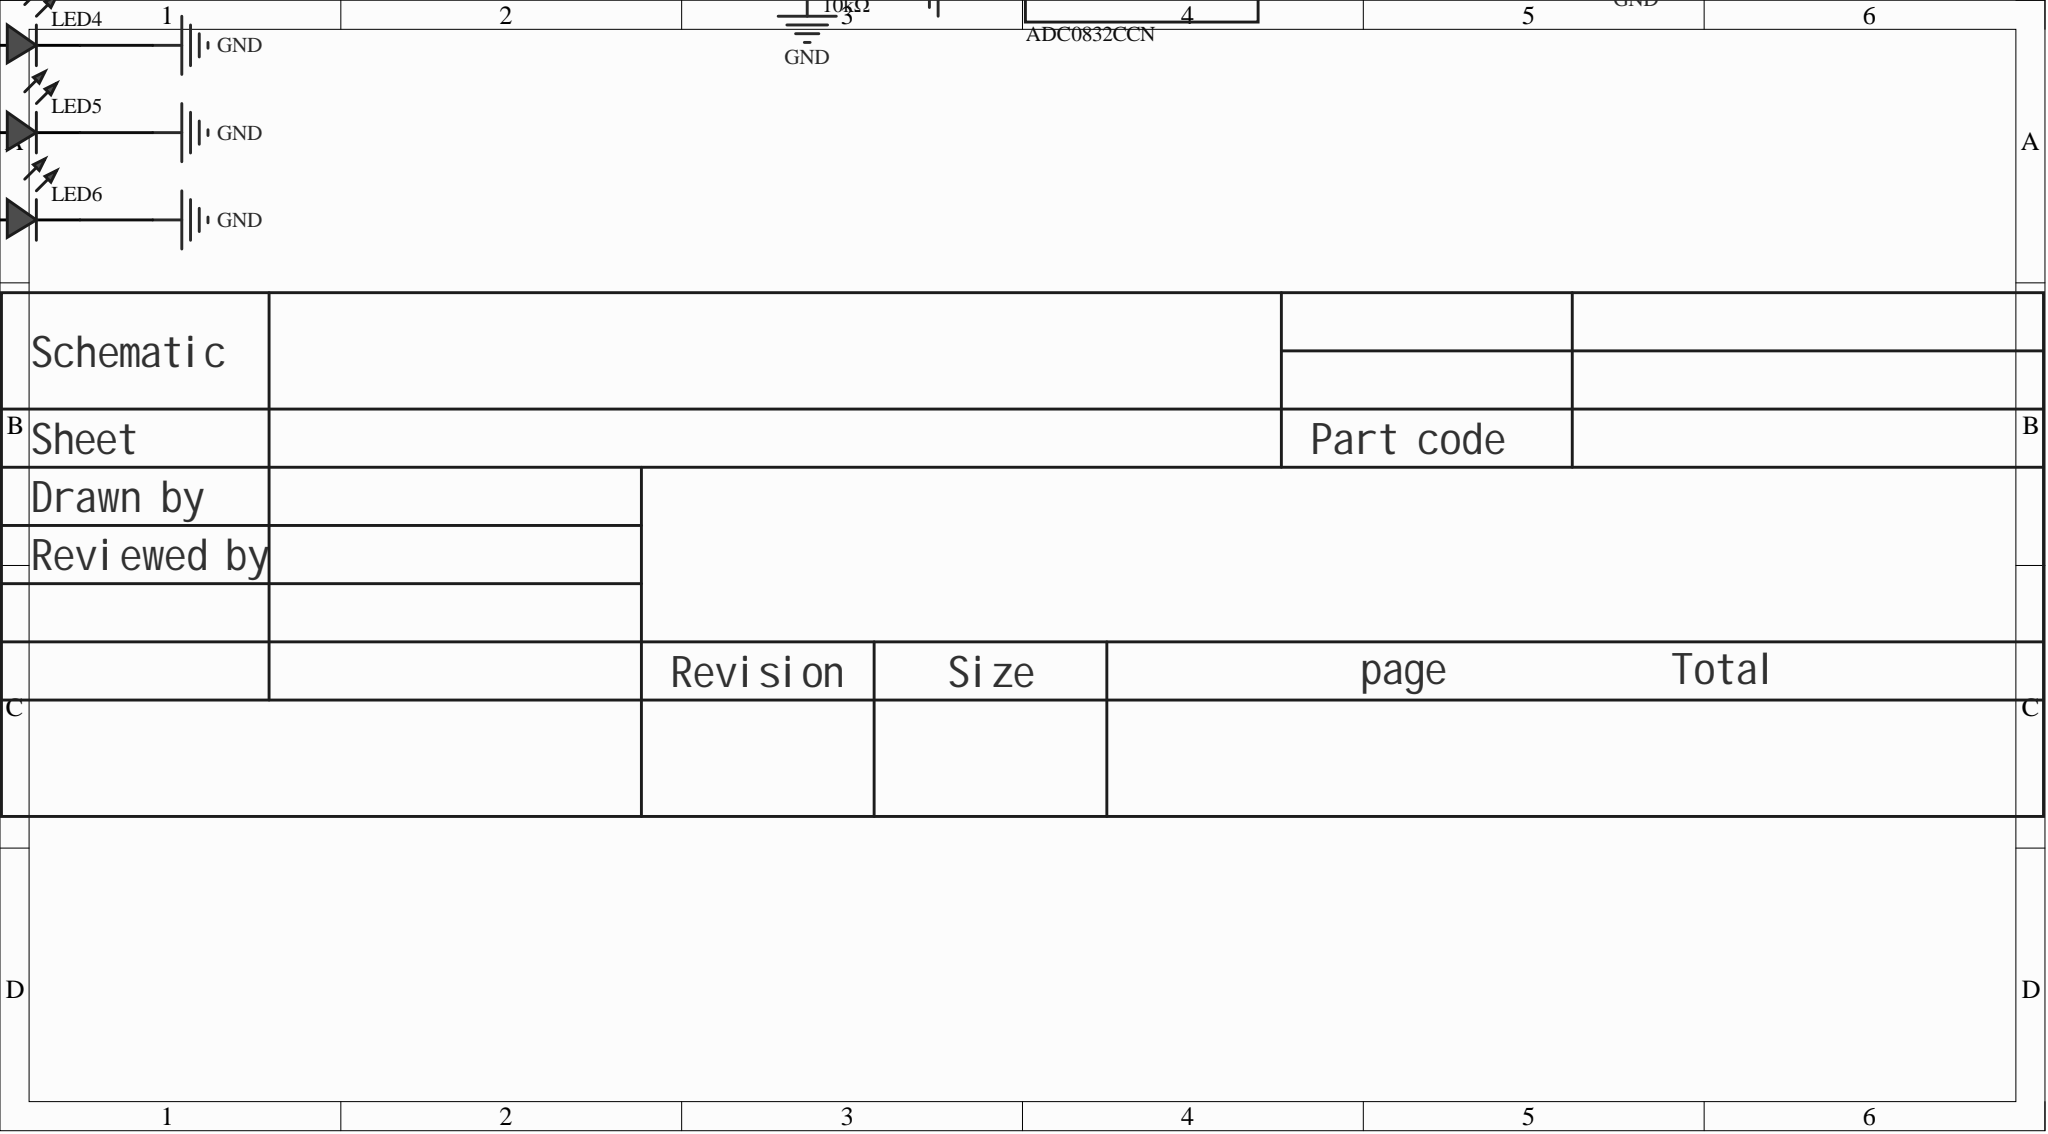Circuit board | Altium Designer | 36 parts | 43 nets
Bill of materials:
Comment,Description,Designator,Footprint,LibRef,Quantity
"buzzer","","BUZZER1","BUZ-TH_BD12.0-P6.00-D0.9-RD","buzzer","1"
"10uF","Capacitance: 10uF; tolerance: ±20%; rated voltage: 250V; ripple current: -; equivalent series resistance: -;","C4","CAP-TH_BD6.3-P2.50-D1.0-FD","LKMC1202E100MF","1"
"30pF","Capacitance: 30pF; tolerance: ±5%; rated voltage: 50V; temperature coefficient: C0G;","C5, C6","CAP-TH_L3.6-W2.3-P5.00-D0.5","K300J10C0GF5UH5","2"
"","","D1","DO_1N4007","D_1N4007A","1"
"","","H1, H2","HDR-TH_2P-P2.54-V-M-1","HDR-M_2.54_1x2P","2"
"","","H3","HDR-TH_6P-P2.54-V-F","HDR-F_2.54_1x6P","1"
"HS1602A","Main control chip: SPLC780; size (inch): 2;","LCD1","LCD1602","HS1602A","1"
"","","LED1, LED2, LED3, LED4, LED5, LED6","LED_TH-3mm","LED_TH-R_3mm","6"
"10kΩ","","PR1","R_3296","R_3296","1"
"","","Q1","S8550P_SOT","S8550_SOT_PNP","1"
"","","Q2","S8050_SOT-23","S8050_SOT_NPN","1"
"10kΩ","","R1, R2, R4, R39","Res_1/8W","Res_AXIAL-1/8W","4"
"1kΩ","","R3","Res_1/8W","Res_AXIAL-1/8W","1"
"2.2kΩ","","R5","Res_1/8W","Res_AXIAL-1/8W","1"
"1K","","R6","R0805","Res_0805","1"
"HT46F-DC12V-SHAG","","RL1","RELAY-TH_HT46F-DCXXV-SHAG","HT46F-DC12V-SHAG","1"
"-","Number of resistors: -; resistance: -; power per element: -;","RN1","RES-ARRAY-TH_9P-P2.54-D1.0","排阻 10 K 5%","1"
"Tact switch, 6*6*5 plastic head, 260G, travel 0.25mm, through-hole 2-pin","","SW1, SW7, SW8, SW9, SW10","KEY-TH_2P-L6.0-W6.0-P5.00","轻触开关,6*6*5塑头,260G,行程0.25mm,直插中2脚","5"
"STC89C52","CPU core: 51 series; program storage: 61KB; total RAM: 1.25KB; GPIO port count: 35; operating voltage: 3.5V~5.5V; CPU max frequency: -; program memory type: FLASH;","U1","DIP-40_L52.3-W13.9-P2.54-LS15.2-BL","STC89C516RD+40I-PDIP40","1"
"12MHz","Frequency: 12MHz; room-temperature frequency tolerance: ±30ppm; external load capacitance: -; frequency stability (full temperature): ±50ppm;","U2","HC-49US_L11.0-W4.6-P4.88","ECS-120-S-4","1"
"DHT11","New capacitive digital temperature and humidity sensor; old model discontinued, 16.1x12.6x5.8mm","U3","SENSOR-TH_DHT11","DHT11","1"
"ADC0832CCN","","U4","DIP-8_L9.7-W6.4-P2.54-LS7.6-BL","ADC0832CCN","1"
Netlist (Protel format):
[
BUZZER1
BUZ-TH_BD12.0-P6.00-D0.9-RD
buzzer



]
[
C4
CAP-TH_BD6.3-P2.50-D1.0-FD
10uF



]
[
C5
CAP-TH_L3.6-W2.3-P5.00-D0.5
30pF



]
[
C6
CAP-TH_L3.6-W2.3-P5.00-D0.5
30pF



]
[
D1
DO_1N4007




]
[
H1
HDR-TH_2P-P2.54-V-M-1




]
[
H2
HDR-TH_2P-P2.54-V-M-1




]
[
H3
HDR-TH_6P-P2.54-V-F




]
[
LCD1
LCD1602
HS1602A



]
[
LED1
LED_TH-3mm




]
[
LED2
LED_TH-3mm




]
[
LED3
LED_TH-3mm




]
[
LED4
LED_TH-3mm




]
[
LED5
LED_TH-3mm




]
[
LED6
LED_TH-3mm




]
[
PR1
R_3296
10kΩ



]
[
Q1
S8550P_SOT




]
[
Q2
S8050_SOT-23




]
[
R1
Res_1/8W
10kΩ



]
[
R2
Res_1/8W
10kΩ



]
[
R3
Res_1/8W
1kΩ



]
[
R4
Res_1/8W
10kΩ



]
[
R5
Res_1/8W
2.2kΩ



]
[
R6
R0805
1K



]
[
R39
Res_1/8W
10kΩ



]
[
RL1
RELAY-TH_HT46F-DCXXV-SHAG
HT46F-DC12V-SHAG



]
[
RN1
RES-ARRAY-TH_9P-P2.54-D1.0
-



]
[
SW1
KEY-TH_2P-L6.0-W6.0-P5.00
Tact switch, 6*6*5 plastic head, 260G, travel 0.25mm, through-hole 2-pin



]
[
SW7
KEY-TH_2P-L6.0-W6.0-P5.00
Tact switch, 6*6*5 plastic head, 260G, travel 0.25mm, through-hole 2-pin



]
[
SW8
KEY-TH_2P-L6.0-W6.0-P5.00
Tact switch, 6*6*5 plastic head, 260G, travel 0.25mm, through-hole 2-pin



]
[
SW9
KEY-TH_2P-L6.0-W6.0-P5.00
Tact switch, 6*6*5 plastic head, 260G, travel 0.25mm, through-hole 2-pin



]
[
SW10
KEY-TH_2P-L6.0-W6.0-P5.00
Tact switch, 6*6*5 plastic head, 260G, travel 0.25mm, through-hole 2-pin



]
[
U1
DIP-40_L52.3-W13.9-P2.54-LS15.2-BL
STC89C52



]
[
U2
HC-49US_L11.0-W4.6-P4.88
12MHz



]
[
U3
SENSOR-TH_DHT11
DHT11



]
[
U4
DIP-8_L9.7-W6.4-P2.54-LS7.6-BL
ADC0832CCN



]
(
VCC
H3-2
LCD1-2
LCD1-15
)
(
RW
LCD1-5
U1-27
)
(
RS
LCD1-4
U1-28
)
(
P12
U1-3
U4-1
)
(
P11
U1-2
U4-5
U4-6
)
(
P10
U1-1
U4-7
)
(
NetSW10_2
SW10-2
U1-4
)
(
NetSW9_2
SW9-2
U1-5
)
(
NetSW8_2
SW8-2
U1-6
)
(
NetSW7_2
SW7-2
U1-7
)
(
NetRN1_9
RN1-9
U1-32
)
(
NetR6_2
R6-2
U1-22
)
(
NetR5_2
R5-2
U1-21
)
(
NetR4_1
R4-1
SW1-2
U1-8
)
(
NetQ2_1
Q2-1
R6-1
)
(
NetQ1_1
Q1-1
R5-1
)
(
NetPR1_2
PR1-2
U4-2
)
(
NetLCD1_14
LCD1-14
RN1-8
U1-33
)
(
NetLCD1_13
LCD1-13
RN1-7
U1-34
)
(
NetLCD1_12
LCD1-12
RN1-6
U1-35
)
(
NetLCD1_11
LCD1-11
RN1-5
U1-36
)
(
NetLCD1_10
LCD1-10
RN1-4
U1-37
)
(
NetLCD1_9
LCD1-9
RN1-3
U1-38
)
(
NetLCD1_8
LCD1-8
RN1-2
U1-39
)
(
NetLCD1_3
LCD1-3
R2-1
R3-2
)
(
NetH3_5
H3-5
U1-11
)
(
NetH3_4
H3-4
U1-10
)
(
NetH1_2
H1-2
RL1-3
)
(
NetD1_2
D1-2
Q2-3
RL1-2
)
(
NetC6_2
C6-2
U1-19
U2-2
)
(
NetC5_2
C5-2
U1-18
U2-1
)
(
NetC4_2
C4-2
R39-2
U1-9
)
(
NetBUZZER1_1
BUZZER1-1
Q1-2
)
(
GND
C5-1
C6-1
H1-1
H2-2
H3-3
LCD1-1
LCD1-16
LED1-2
LED2-2
LED3-2
LED4-2
LED5-2
LED6-2
PR1-1
Q1-3
Q2-2
R3-1
R39-1
SW1-1
SW7-1
SW8-1
SW9-1
SW10-1
U1-20
U3-4
U4-4
)
(
EN
LCD1-6
U1-26
)
(
+5V
BUZZER1-2
C4-1
D1-1
H2-1
LCD1-7
PR1-3
R1-2
R2-2
R4-2
RL1-1
RL1-4
RN1-1
U1-40
U3-1
U4-8
)
(
37
R1-1
U1-17
U3-2
)
(
36
LED6-1
U1-16
)
(
35
LED5-1
U1-15
)
(
34
LED4-1
U1-14
)
(
33
LED3-1
U1-13
)
(
32
LED2-1
U1-12
)
(
31
LED1-1
U1-23
)